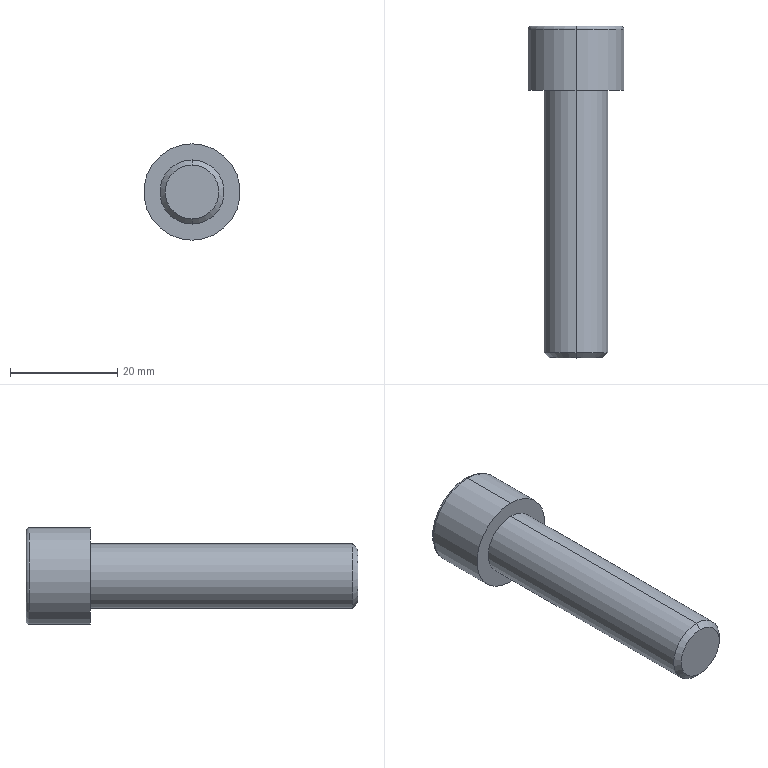Part | SolidWorks | features BaseBody 1 | 1 solid | 18 faces | box 18 x 62 x 18 mm | volume 8155 mm3 | plane 10 | cylinder 4 | cone 2 | torus 2 | commonest cylinder face diameters 12 x2 18 x2
STEP:
#1=CARTESIAN_POINT('',(0.,-50.,-5.035));
#2=VERTEX_POINT('',#1);
#3=CARTESIAN_POINT('',(0.,-50.,5.035));
#4=VERTEX_POINT('',#3);
#5=CARTESIAN_POINT('',(0.,-50.,0.));
#6=DIRECTION('',(0.,-1.,0.));
#7=DIRECTION('',(0.,0.,-1.));
#8=AXIS2_PLACEMENT_3D('',#5,#6,#7);
#9=CIRCLE('',#8,5.035);
#10=EDGE_CURVE('',#2,#4,#9,.T.);
#11=ORIENTED_EDGE('',*,*,#10,.F.);
#12=CARTESIAN_POINT('',(0.,-49.035,-6.));
#13=VERTEX_POINT('',#12);
#14=CARTESIAN_POINT('',(0.,-50.,-5.035));
#15=DIRECTION('',(0.,0.7071,-0.7071));
#16=VECTOR('',#15,1000.);
#17=LINE('',#14,#16);
#18=EDGE_CURVE('',#2,#13,#17,.T.);
#19=ORIENTED_EDGE('',*,*,#18,.T.);
#20=CARTESIAN_POINT('',(0.,-49.035,6.));
#21=VERTEX_POINT('',#20);
#22=CARTESIAN_POINT('',(0.,-49.035,0.));
#23=DIRECTION('',(0.,1.,0.));
#24=DIRECTION('',(0.,0.,-1.));
#25=AXIS2_PLACEMENT_3D('',#22,#23,#24);
#26=CIRCLE('',#25,6.);
#27=EDGE_CURVE('',#21,#13,#26,.T.);
#28=ORIENTED_EDGE('',*,*,#27,.F.);
#29=CARTESIAN_POINT('',(0.,-50.,5.035));
#30=DIRECTION('',(0.,0.7071,0.7071));
#31=VECTOR('',#30,1000.);
#32=LINE('',#29,#31);
#33=EDGE_CURVE('',#4,#21,#32,.T.);
#34=ORIENTED_EDGE('',*,*,#33,.F.);
#35=EDGE_LOOP('',(#11,#19,#28,#34));
#36=FACE_OUTER_BOUND('',#35,.T.);
#37=CARTESIAN_POINT('',(0.,-50.,0.));
#38=DIRECTION('',(0.,1.,0.));
#39=DIRECTION('',(0.,0.,1.));
#40=AXIS2_PLACEMENT_3D('',#37,#38,#39);
#41=CONICAL_SURFACE('',#40,5.035,0.7854);
#42=ADVANCED_FACE('',(#36),#41,.T.);
#43=ORIENTED_EDGE('',*,*,#27,.T.);
#44=CARTESIAN_POINT('',(0.,0.,-6.));
#45=VERTEX_POINT('',#44);
#46=CARTESIAN_POINT('',(0.,-50.,-6.));
#47=DIRECTION('',(0.,1.,0.));
#48=VECTOR('',#47,1000.);
#49=LINE('',#46,#48);
#50=EDGE_CURVE('',#13,#45,#49,.T.);
#51=ORIENTED_EDGE('',*,*,#50,.T.);
#52=CARTESIAN_POINT('',(0.,0.,6.));
#53=VERTEX_POINT('',#52);
#54=CARTESIAN_POINT('',(0.,0.,0.));
#55=DIRECTION('',(0.,-1.,0.));
#56=DIRECTION('',(0.,0.,1.));
#57=AXIS2_PLACEMENT_3D('',#54,#55,#56);
#58=CIRCLE('',#57,6.);
#59=EDGE_CURVE('',#45,#53,#58,.T.);
#60=ORIENTED_EDGE('',*,*,#59,.T.);
#61=CARTESIAN_POINT('',(0.,-50.,6.));
#62=DIRECTION('',(0.,1.,0.));
#63=VECTOR('',#62,1000.);
#64=LINE('',#61,#63);
#65=EDGE_CURVE('',#21,#53,#64,.T.);
#66=ORIENTED_EDGE('',*,*,#65,.F.);
#67=EDGE_LOOP('',(#43,#51,#60,#66));
#68=FACE_OUTER_BOUND('',#67,.T.);
#69=CARTESIAN_POINT('',(0.,-50.,0.));
#70=DIRECTION('',(0.,1.,0.));
#71=DIRECTION('',(0.,0.,1.));
#72=AXIS2_PLACEMENT_3D('',#69,#70,#71);
#73=CYLINDRICAL_SURFACE('',#72,6.);
#74=ADVANCED_FACE('',(#68),#73,.T.);
#75=CARTESIAN_POINT('',(0.,11.4,-9.));
#76=VERTEX_POINT('',#75);
#77=CARTESIAN_POINT('',(0.,11.4,9.));
#78=VERTEX_POINT('',#77);
#79=CARTESIAN_POINT('',(0.,11.4,0.));
#80=DIRECTION('',(0.,-1.,0.));
#81=DIRECTION('',(0.,0.,1.));
#82=AXIS2_PLACEMENT_3D('',#79,#80,#81);
#83=CIRCLE('',#82,9.);
#84=EDGE_CURVE('',#76,#78,#83,.T.);
#85=ORIENTED_EDGE('',*,*,#84,.F.);
#86=CARTESIAN_POINT('',(0.,12.,-8.4));
#87=VERTEX_POINT('',#86);
#88=CARTESIAN_POINT('',(0.,11.4,-8.4));
#89=DIRECTION('',(1.,0.,0.));
#90=DIRECTION('',(0.,0.,-1.));
#91=AXIS2_PLACEMENT_3D('',#88,#89,#90);
#92=CIRCLE('',#91,0.6);
#93=EDGE_CURVE('',#76,#87,#92,.T.);
#94=ORIENTED_EDGE('',*,*,#93,.T.);
#95=CARTESIAN_POINT('',(0.,12.,8.4));
#96=VERTEX_POINT('',#95);
#97=CARTESIAN_POINT('',(0.,12.,0.));
#98=DIRECTION('',(0.,1.,0.));
#99=DIRECTION('',(0.,0.,1.));
#100=AXIS2_PLACEMENT_3D('',#97,#98,#99);
#101=CIRCLE('',#100,8.4);
#102=EDGE_CURVE('',#96,#87,#101,.T.);
#103=ORIENTED_EDGE('',*,*,#102,.F.);
#104=CARTESIAN_POINT('',(0.,11.4,8.4));
#105=DIRECTION('',(-1.,0.,0.));
#106=DIRECTION('',(0.,0.,1.));
#107=AXIS2_PLACEMENT_3D('',#104,#105,#106);
#108=CIRCLE('',#107,0.6);
#109=EDGE_CURVE('',#78,#96,#108,.T.);
#110=ORIENTED_EDGE('',*,*,#109,.F.);
#111=EDGE_LOOP('',(#85,#94,#103,#110));
#112=FACE_OUTER_BOUND('',#111,.T.);
#113=CARTESIAN_POINT('',(0.,11.4,0.));
#114=DIRECTION('',(0.,1.,0.));
#115=DIRECTION('',(0.,0.,1.));
#116=AXIS2_PLACEMENT_3D('',#113,#114,#115);
#117=TOROIDAL_SURFACE('',#116,8.4,0.6);
#118=ADVANCED_FACE('',(#112),#117,.T.);
#119=ORIENTED_EDGE('',*,*,#84,.T.);
#120=CARTESIAN_POINT('',(0.,0.,9.));
#121=VERTEX_POINT('',#120);
#122=CARTESIAN_POINT('',(0.,12.,9.));
#123=DIRECTION('',(0.,-1.,0.));
#124=VECTOR('',#123,1000.);
#125=LINE('',#122,#124);
#126=EDGE_CURVE('',#78,#121,#125,.T.);
#127=ORIENTED_EDGE('',*,*,#126,.T.);
#128=CARTESIAN_POINT('',(0.,0.,-9.));
#129=VERTEX_POINT('',#128);
#130=CARTESIAN_POINT('',(0.,0.,0.));
#131=DIRECTION('',(0.,1.,0.));
#132=DIRECTION('',(0.,0.,1.));
#133=AXIS2_PLACEMENT_3D('',#130,#131,#132);
#134=CIRCLE('',#133,9.);
#135=EDGE_CURVE('',#121,#129,#134,.T.);
#136=ORIENTED_EDGE('',*,*,#135,.T.);
#137=CARTESIAN_POINT('',(0.,12.,-9.));
#138=DIRECTION('',(0.,-1.,0.));
#139=VECTOR('',#138,1000.);
#140=LINE('',#137,#139);
#141=EDGE_CURVE('',#76,#129,#140,.T.);
#142=ORIENTED_EDGE('',*,*,#141,.F.);
#143=EDGE_LOOP('',(#119,#127,#136,#142));
#144=FACE_OUTER_BOUND('',#143,.T.);
#145=CARTESIAN_POINT('',(0.,12.,0.));
#146=DIRECTION('',(0.,-1.,0.));
#147=DIRECTION('',(0.,0.,-1.));
#148=AXIS2_PLACEMENT_3D('',#145,#146,#147);
#149=CYLINDRICAL_SURFACE('',#148,9.);
#150=ADVANCED_FACE('',(#144),#149,.T.);
#151=CARTESIAN_POINT('',(0.,-50.,0.));
#152=DIRECTION('',(0.,-1.,0.));
#153=DIRECTION('',(0.,0.,-1.));
#154=AXIS2_PLACEMENT_3D('',#151,#152,#153);
#155=CIRCLE('',#154,5.035);
#156=EDGE_CURVE('',#4,#2,#155,.T.);
#157=ORIENTED_EDGE('',*,*,#156,.T.);
#158=ORIENTED_EDGE('',*,*,#10,.T.);
#159=EDGE_LOOP('',(#157,#158));
#160=FACE_OUTER_BOUND('',#159,.T.);
#161=CARTESIAN_POINT('',(0.,-50.,0.));
#162=DIRECTION('',(0.,-1.,0.));
#163=DIRECTION('',(0.,0.,-1.));
#164=AXIS2_PLACEMENT_3D('',#161,#162,#163);
#165=PLANE('',#164);
#166=ADVANCED_FACE('',(#160),#165,.T.);
#167=CARTESIAN_POINT('',(2.921,6.,5.06));
#168=VERTEX_POINT('',#167);
#169=CARTESIAN_POINT('',(5.843,6.,0.));
#170=VERTEX_POINT('',#169);
#171=CARTESIAN_POINT('',(2.921,6.,5.06));
#172=DIRECTION('',(0.5,0.,-0.866));
#173=VECTOR('',#172,1000.);
#174=LINE('',#171,#173);
#175=EDGE_CURVE('',#168,#170,#174,.T.);
#176=ORIENTED_EDGE('',*,*,#175,.T.);
#177=CARTESIAN_POINT('',(2.921,6.,-5.06));
#178=VERTEX_POINT('',#177);
#179=CARTESIAN_POINT('',(5.843,6.,0.));
#180=DIRECTION('',(-0.5,0.,-0.866));
#181=VECTOR('',#180,1000.);
#182=LINE('',#179,#181);
#183=EDGE_CURVE('',#170,#178,#182,.T.);
#184=ORIENTED_EDGE('',*,*,#183,.T.);
#185=CARTESIAN_POINT('',(-2.921,6.,-5.06));
#186=VERTEX_POINT('',#185);
#187=CARTESIAN_POINT('',(2.921,6.,-5.06));
#188=DIRECTION('',(-1.,0.,0.));
#189=VECTOR('',#188,1000.);
#190=LINE('',#187,#189);
#191=EDGE_CURVE('',#178,#186,#190,.T.);
#192=ORIENTED_EDGE('',*,*,#191,.T.);
#193=CARTESIAN_POINT('',(-5.843,6.,0.));
#194=VERTEX_POINT('',#193);
#195=CARTESIAN_POINT('',(-2.921,6.,-5.06));
#196=DIRECTION('',(-0.5,0.,0.866));
#197=VECTOR('',#196,1000.);
#198=LINE('',#195,#197);
#199=EDGE_CURVE('',#186,#194,#198,.T.);
#200=ORIENTED_EDGE('',*,*,#199,.T.);
#201=CARTESIAN_POINT('',(-2.921,6.,5.06));
#202=VERTEX_POINT('',#201);
#203=CARTESIAN_POINT('',(-5.843,6.,0.));
#204=DIRECTION('',(0.5,0.,0.866));
#205=VECTOR('',#204,1000.);
#206=LINE('',#203,#205);
#207=EDGE_CURVE('',#194,#202,#206,.T.);
#208=ORIENTED_EDGE('',*,*,#207,.T.);
#209=CARTESIAN_POINT('',(-2.921,6.,5.06));
#210=DIRECTION('',(1.,0.,0.));
#211=VECTOR('',#210,1000.);
#212=LINE('',#209,#211);
#213=EDGE_CURVE('',#202,#168,#212,.T.);
#214=ORIENTED_EDGE('',*,*,#213,.T.);
#215=EDGE_LOOP('',(#176,#184,#192,#200,#208,#214));
#216=FACE_OUTER_BOUND('',#215,.T.);
#217=CARTESIAN_POINT('',(0.,6.,0.));
#218=DIRECTION('',(0.,1.,0.));
#219=DIRECTION('',(1.,0.,0.));
#220=AXIS2_PLACEMENT_3D('',#217,#218,#219);
#221=PLANE('',#220);
#222=ADVANCED_FACE('',(#216),#221,.T.);
#223=CARTESIAN_POINT('',(5.843,12.,0.));
#224=VERTEX_POINT('',#223);
#225=CARTESIAN_POINT('',(2.921,12.,-5.06));
#226=VERTEX_POINT('',#225);
#227=CARTESIAN_POINT('',(5.843,12.,0.));
#228=DIRECTION('',(-0.5,0.,-0.866));
#229=VECTOR('',#228,1000.);
#230=LINE('',#227,#229);
#231=EDGE_CURVE('',#224,#226,#230,.T.);
#232=ORIENTED_EDGE('',*,*,#231,.T.);
#233=CARTESIAN_POINT('',(2.921,6.,-5.06));
#234=DIRECTION('',(0.,1.,0.));
#235=VECTOR('',#234,1000.);
#236=LINE('',#233,#235);
#237=EDGE_CURVE('',#178,#226,#236,.T.);
#238=ORIENTED_EDGE('',*,*,#237,.F.);
#239=ORIENTED_EDGE('',*,*,#183,.F.);
#240=CARTESIAN_POINT('',(5.843,6.,0.));
#241=DIRECTION('',(0.,1.,0.));
#242=VECTOR('',#241,1000.);
#243=LINE('',#240,#242);
#244=EDGE_CURVE('',#170,#224,#243,.T.);
#245=ORIENTED_EDGE('',*,*,#244,.T.);
#246=EDGE_LOOP('',(#232,#238,#239,#245));
#247=FACE_OUTER_BOUND('',#246,.T.);
#248=CARTESIAN_POINT('',(5.843,6.,0.));
#249=DIRECTION('',(0.866,0.,-0.5));
#250=DIRECTION('',(0.,-1.,0.));
#251=AXIS2_PLACEMENT_3D('',#248,#249,#250);
#252=PLANE('',#251);
#253=ADVANCED_FACE('',(#247),#252,.F.);
#254=CARTESIAN_POINT('',(-2.921,12.,-5.06));
#255=VERTEX_POINT('',#254);
#256=CARTESIAN_POINT('',(2.921,12.,-5.06));
#257=DIRECTION('',(-1.,0.,0.));
#258=VECTOR('',#257,1000.);
#259=LINE('',#256,#258);
#260=EDGE_CURVE('',#226,#255,#259,.T.);
#261=ORIENTED_EDGE('',*,*,#260,.T.);
#262=CARTESIAN_POINT('',(-2.921,6.,-5.06));
#263=DIRECTION('',(0.,1.,0.));
#264=VECTOR('',#263,1000.);
#265=LINE('',#262,#264);
#266=EDGE_CURVE('',#186,#255,#265,.T.);
#267=ORIENTED_EDGE('',*,*,#266,.F.);
#268=ORIENTED_EDGE('',*,*,#191,.F.);
#269=ORIENTED_EDGE('',*,*,#237,.T.);
#270=EDGE_LOOP('',(#261,#267,#268,#269));
#271=FACE_OUTER_BOUND('',#270,.T.);
#272=CARTESIAN_POINT('',(2.921,6.,-5.06));
#273=DIRECTION('',(0.,0.,-1.));
#274=DIRECTION('',(0.,-1.,0.));
#275=AXIS2_PLACEMENT_3D('',#272,#273,#274);
#276=PLANE('',#275);
#277=ADVANCED_FACE('',(#271),#276,.F.);
#278=CARTESIAN_POINT('',(-5.843,12.,0.));
#279=VERTEX_POINT('',#278);
#280=CARTESIAN_POINT('',(-2.921,12.,-5.06));
#281=DIRECTION('',(-0.5,0.,0.866));
#282=VECTOR('',#281,1000.);
#283=LINE('',#280,#282);
#284=EDGE_CURVE('',#255,#279,#283,.T.);
#285=ORIENTED_EDGE('',*,*,#284,.T.);
#286=CARTESIAN_POINT('',(-5.843,6.,0.));
#287=DIRECTION('',(0.,1.,0.));
#288=VECTOR('',#287,1000.);
#289=LINE('',#286,#288);
#290=EDGE_CURVE('',#194,#279,#289,.T.);
#291=ORIENTED_EDGE('',*,*,#290,.F.);
#292=ORIENTED_EDGE('',*,*,#199,.F.);
#293=ORIENTED_EDGE('',*,*,#266,.T.);
#294=EDGE_LOOP('',(#285,#291,#292,#293));
#295=FACE_OUTER_BOUND('',#294,.T.);
#296=CARTESIAN_POINT('',(-2.921,6.,-5.06));
#297=DIRECTION('',(-0.866,0.,-0.5));
#298=DIRECTION('',(-0.5,0.,0.866));
#299=AXIS2_PLACEMENT_3D('',#296,#297,#298);
#300=PLANE('',#299);
#301=ADVANCED_FACE('',(#295),#300,.F.);
#302=CARTESIAN_POINT('',(-2.921,12.,5.06));
#303=VERTEX_POINT('',#302);
#304=CARTESIAN_POINT('',(-5.843,12.,0.));
#305=DIRECTION('',(0.5,0.,0.866));
#306=VECTOR('',#305,1000.);
#307=LINE('',#304,#306);
#308=EDGE_CURVE('',#279,#303,#307,.T.);
#309=ORIENTED_EDGE('',*,*,#308,.T.);
#310=CARTESIAN_POINT('',(-2.921,6.,5.06));
#311=DIRECTION('',(0.,1.,0.));
#312=VECTOR('',#311,1000.);
#313=LINE('',#310,#312);
#314=EDGE_CURVE('',#202,#303,#313,.T.);
#315=ORIENTED_EDGE('',*,*,#314,.F.);
#316=ORIENTED_EDGE('',*,*,#207,.F.);
#317=ORIENTED_EDGE('',*,*,#290,.T.);
#318=EDGE_LOOP('',(#309,#315,#316,#317));
#319=FACE_OUTER_BOUND('',#318,.T.);
#320=CARTESIAN_POINT('',(-5.843,6.,0.));
#321=DIRECTION('',(-0.866,0.,0.5));
#322=DIRECTION('',(0.,1.,0.));
#323=AXIS2_PLACEMENT_3D('',#320,#321,#322);
#324=PLANE('',#323);
#325=ADVANCED_FACE('',(#319),#324,.F.);
#326=CARTESIAN_POINT('',(2.921,12.,5.06));
#327=VERTEX_POINT('',#326);
#328=CARTESIAN_POINT('',(-2.921,12.,5.06));
#329=DIRECTION('',(1.,0.,0.));
#330=VECTOR('',#329,1000.);
#331=LINE('',#328,#330);
#332=EDGE_CURVE('',#303,#327,#331,.T.);
#333=ORIENTED_EDGE('',*,*,#332,.T.);
#334=CARTESIAN_POINT('',(2.921,6.,5.06));
#335=DIRECTION('',(0.,1.,0.));
#336=VECTOR('',#335,1000.);
#337=LINE('',#334,#336);
#338=EDGE_CURVE('',#168,#327,#337,.T.);
#339=ORIENTED_EDGE('',*,*,#338,.F.);
#340=ORIENTED_EDGE('',*,*,#213,.F.);
#341=ORIENTED_EDGE('',*,*,#314,.T.);
#342=EDGE_LOOP('',(#333,#339,#340,#341));
#343=FACE_OUTER_BOUND('',#342,.T.);
#344=CARTESIAN_POINT('',(-2.921,6.,5.06));
#345=DIRECTION('',(0.,0.,1.));
#346=DIRECTION('',(1.,0.,0.));
#347=AXIS2_PLACEMENT_3D('',#344,#345,#346);
#348=PLANE('',#347);
#349=ADVANCED_FACE('',(#343),#348,.F.);
#350=CARTESIAN_POINT('',(2.921,12.,5.06));
#351=DIRECTION('',(0.5,0.,-0.866));
#352=VECTOR('',#351,1000.);
#353=LINE('',#350,#352);
#354=EDGE_CURVE('',#327,#224,#353,.T.);
#355=ORIENTED_EDGE('',*,*,#354,.T.);
#356=ORIENTED_EDGE('',*,*,#244,.F.);
#357=ORIENTED_EDGE('',*,*,#175,.F.);
#358=ORIENTED_EDGE('',*,*,#338,.T.);
#359=EDGE_LOOP('',(#355,#356,#357,#358));
#360=FACE_OUTER_BOUND('',#359,.T.);
#361=CARTESIAN_POINT('',(2.921,6.,5.06));
#362=DIRECTION('',(0.866,0.,0.5));
#363=DIRECTION('',(0.,-1.,0.));
#364=AXIS2_PLACEMENT_3D('',#361,#362,#363);
#365=PLANE('',#364);
#366=ADVANCED_FACE('',(#360),#365,.F.);
#367=ORIENTED_EDGE('',*,*,#354,.F.);
#368=ORIENTED_EDGE('',*,*,#332,.F.);
#369=ORIENTED_EDGE('',*,*,#308,.F.);
#370=ORIENTED_EDGE('',*,*,#284,.F.);
#371=ORIENTED_EDGE('',*,*,#260,.F.);
#372=ORIENTED_EDGE('',*,*,#231,.F.);
#373=EDGE_LOOP('',(#367,#368,#369,#370,#371,#372));
#374=FACE_BOUND('',#373,.T.);
#375=ORIENTED_EDGE('',*,*,#102,.T.);
#376=CARTESIAN_POINT('',(0.,12.,0.));
#377=DIRECTION('',(0.,1.,0.));
#378=DIRECTION('',(0.,0.,1.));
#379=AXIS2_PLACEMENT_3D('',#376,#377,#378);
#380=CIRCLE('',#379,8.4);
#381=EDGE_CURVE('',#87,#96,#380,.T.);
#382=ORIENTED_EDGE('',*,*,#381,.T.);
#383=EDGE_LOOP('',(#375,#382));
#384=FACE_OUTER_BOUND('',#383,.T.);
#385=CARTESIAN_POINT('',(0.,12.,0.));
#386=DIRECTION('',(0.,1.,0.));
#387=DIRECTION('',(1.,0.,0.));
#388=AXIS2_PLACEMENT_3D('',#385,#386,#387);
#389=PLANE('',#388);
#390=ADVANCED_FACE('',(#374,#384),#389,.T.);
#391=CARTESIAN_POINT('',(0.,0.,0.));
#392=DIRECTION('',(0.,-1.,0.));
#393=DIRECTION('',(0.,0.,1.));
#394=AXIS2_PLACEMENT_3D('',#391,#392,#393);
#395=CIRCLE('',#394,6.);
#396=EDGE_CURVE('',#53,#45,#395,.T.);
#397=ORIENTED_EDGE('',*,*,#396,.F.);
#398=ORIENTED_EDGE('',*,*,#59,.F.);
#399=EDGE_LOOP('',(#397,#398));
#400=FACE_BOUND('',#399,.T.);
#401=CARTESIAN_POINT('',(0.,0.,0.));
#402=DIRECTION('',(0.,1.,0.));
#403=DIRECTION('',(0.,0.,1.));
#404=AXIS2_PLACEMENT_3D('',#401,#402,#403);
#405=CIRCLE('',#404,9.);
#406=EDGE_CURVE('',#129,#121,#405,.T.);
#407=ORIENTED_EDGE('',*,*,#406,.F.);
#408=ORIENTED_EDGE('',*,*,#135,.F.);
#409=EDGE_LOOP('',(#407,#408));
#410=FACE_OUTER_BOUND('',#409,.T.);
#411=CARTESIAN_POINT('',(0.,0.,0.));
#412=DIRECTION('',(0.,1.,0.));
#413=DIRECTION('',(1.,0.,0.));
#414=AXIS2_PLACEMENT_3D('',#411,#412,#413);
#415=PLANE('',#414);
#416=ADVANCED_FACE('',(#400,#410),#415,.F.);
#417=ORIENTED_EDGE('',*,*,#126,.F.);
#418=CARTESIAN_POINT('',(0.,11.4,0.));
#419=DIRECTION('',(0.,-1.,0.));
#420=DIRECTION('',(0.,0.,1.));
#421=AXIS2_PLACEMENT_3D('',#418,#419,#420);
#422=CIRCLE('',#421,9.);
#423=EDGE_CURVE('',#78,#76,#422,.T.);
#424=ORIENTED_EDGE('',*,*,#423,.T.);
#425=ORIENTED_EDGE('',*,*,#141,.T.);
#426=ORIENTED_EDGE('',*,*,#406,.T.);
#427=EDGE_LOOP('',(#417,#424,#425,#426));
#428=FACE_OUTER_BOUND('',#427,.T.);
#429=CARTESIAN_POINT('',(0.,12.,0.));
#430=DIRECTION('',(0.,-1.,0.));
#431=DIRECTION('',(0.,0.,-1.));
#432=AXIS2_PLACEMENT_3D('',#429,#430,#431);
#433=CYLINDRICAL_SURFACE('',#432,9.);
#434=ADVANCED_FACE('',(#428),#433,.T.);
#435=ORIENTED_EDGE('',*,*,#93,.F.);
#436=ORIENTED_EDGE('',*,*,#423,.F.);
#437=ORIENTED_EDGE('',*,*,#109,.T.);
#438=ORIENTED_EDGE('',*,*,#381,.F.);
#439=EDGE_LOOP('',(#435,#436,#437,#438));
#440=FACE_OUTER_BOUND('',#439,.T.);
#441=CARTESIAN_POINT('',(0.,11.4,0.));
#442=DIRECTION('',(0.,1.,0.));
#443=DIRECTION('',(0.,0.,1.));
#444=AXIS2_PLACEMENT_3D('',#441,#442,#443);
#445=TOROIDAL_SURFACE('',#444,8.4,0.6);
#446=ADVANCED_FACE('',(#440),#445,.T.);
#447=ORIENTED_EDGE('',*,*,#50,.F.);
#448=CARTESIAN_POINT('',(0.,-49.035,0.));
#449=DIRECTION('',(0.,1.,0.));
#450=DIRECTION('',(0.,0.,-1.));
#451=AXIS2_PLACEMENT_3D('',#448,#449,#450);
#452=CIRCLE('',#451,6.);
#453=EDGE_CURVE('',#13,#21,#452,.T.);
#454=ORIENTED_EDGE('',*,*,#453,.T.);
#455=ORIENTED_EDGE('',*,*,#65,.T.);
#456=ORIENTED_EDGE('',*,*,#396,.T.);
#457=EDGE_LOOP('',(#447,#454,#455,#456));
#458=FACE_OUTER_BOUND('',#457,.T.);
#459=CARTESIAN_POINT('',(0.,-50.,0.));
#460=DIRECTION('',(0.,1.,0.));
#461=DIRECTION('',(0.,0.,1.));
#462=AXIS2_PLACEMENT_3D('',#459,#460,#461);
#463=CYLINDRICAL_SURFACE('',#462,6.);
#464=ADVANCED_FACE('',(#458),#463,.T.);
#465=ORIENTED_EDGE('',*,*,#18,.F.);
#466=ORIENTED_EDGE('',*,*,#156,.F.);
#467=ORIENTED_EDGE('',*,*,#33,.T.);
#468=ORIENTED_EDGE('',*,*,#453,.F.);
#469=EDGE_LOOP('',(#465,#466,#467,#468));
#470=FACE_OUTER_BOUND('',#469,.T.);
#471=CARTESIAN_POINT('',(0.,-50.,0.));
#472=DIRECTION('',(0.,1.,0.));
#473=DIRECTION('',(0.,0.,1.));
#474=AXIS2_PLACEMENT_3D('',#471,#472,#473);
#475=CONICAL_SURFACE('',#474,5.035,0.7854);
#476=ADVANCED_FACE('',(#470),#475,.T.);
#477=CLOSED_SHELL('',(#42,#74,#118,#150,#166,#222,#253,#277,#301,#325,#349,#366,#390,#416,#434,#446,#464,#476));
#478=MANIFOLD_SOLID_BREP('',#477);
#479=CARTESIAN_POINT('',(0.,0.,0.));
#480=DIRECTION('',(0.,0.,1.));
#481=DIRECTION('',(1.,0.,0.));
#482=AXIS2_PLACEMENT_3D('',#479,#480,#481);
#483=(LENGTH_UNIT()NAMED_UNIT(*)SI_UNIT(.MILLI.,.METRE.));
#484=UNCERTAINTY_MEASURE_WITH_UNIT(LENGTH_MEASURE(0.00001),#483,'','');
#485=(NAMED_UNIT(*)PLANE_ANGLE_UNIT()SI_UNIT($,.RADIAN.));
#486=(NAMED_UNIT(*)SI_UNIT($,.STERADIAN.)SOLID_ANGLE_UNIT());
#487=(GEOMETRIC_REPRESENTATION_CONTEXT(3)GLOBAL_UNCERTAINTY_ASSIGNED_CONTEXT((#484))GLOBAL_UNIT_ASSIGNED_CONTEXT((#483,#485,#486))REPRESENTATION_CONTEXT('',''));
#488=ADVANCED_BREP_SHAPE_REPRESENTATION('',(#478,#482),#487);